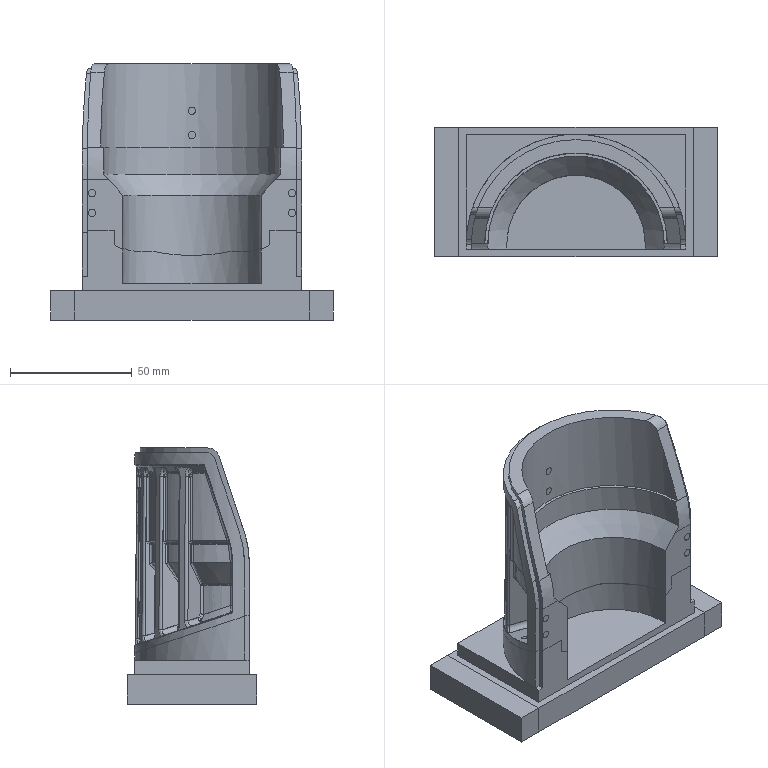NC program | NX | posted by the shop | part box 116 x 53 x 105 mm
Lines 66720 to 68720 of 572762:
T16 M6
;(T16:J-D16  D=16. R=0.)
;(XY=0.2mm Z=0.2mm)
G54 G90 D1
G0 A0.0 C=DC(0.0)
CYCLE832(0.32,_ROUGH,1.)
G0 X-53.306 Y-11.726 S4000 M3 M8
Z3.4
Z.476
G1 Z0.0 F500.
X-50.36 Y-12.824
X-47.214 Y-13.0429
X-44.118 Y-12.441
X-41.284 Y-11.058
X-38.905 Y-8.988
X-37.214 Y-6.338
X-35.878 Y-3.513
X-34.337 Y-.794
X-32.599 Y1.802
X-29.645 Y5.522
X-26.241 Y8.84
X-22.469 Y11.732
X-18.382 Y14.157
X-14.036 Y16.0824
X-9.493 Y17.48
X-4.817 Y18.331
X-.073 Y18.622
X4.672 Y18.351
X9.352 Y17.52
X13.9 Y16.141
X18.254 Y14.235
X22.352 Y11.826
X26.136 Y8.95
X29.553 Y5.647
X32.556 Y1.963
X35.067 Y-2.07
X37.226 Y-6.338
X38.933 Y-8.978
X41.325 Y-11.033
X44.167 Y-12.399
X47.266 Y-12.9826
X50.411 Y-12.744
X53.35 Y-11.629
Z.468
G0 Z3.4
CYCLE832()
;(T16:J-D16  D=16. R=0.)
;(XY=0.3mm Z=0.mm)
SUPA G0 Z-1. D0
SUPA G0 X-1.0 Y-1.0
G54 G90 D1
CYCLE832(0.04,_TOP_SURFACE_SMOOTH_ON+_ORI_SEMIFIN,1.)
TRAFOOF
CYCLE800(0,"AFMING",100000,57,0.,0.,0.,90.,-0.,-180.,0.,0.,0.,-1,100.,1)
G0 X-62.6 Y84.699 S4000 M3
Z102.5121
X-62.6 Y84.699 Z102.5121
Z23.5
G1 X-53. F500.
X53.
Y79.
X50.753 Y76.997
X-50.753
Y69.295
X50.753
Y61.593
X-50.753
Y53.891
X50.753
X60.353
G0 Z102.5121
CYCLE800()
CYCLE832()
;(T16:J-D16  D=16. R=0.)
;(XY=0.3mm Z=0.mm)
SUPA G0 Z-1. D0
SUPA G0 X-1.0 Y-1.0
G54 G90 D1
CYCLE832(0.04,_TOP_SURFACE_SMOOTH_ON+_ORI_SEMIFIN,1.)
TRAFOOF
CYCLE800(0,"AFMING",100000,57,0.,0.,0.,-90.,0.,-0.,0.,0.,0.,-1,100.,1)
G0 X62.6 Y79.001 S4000 M3
Z102.4879
X62.6 Y79.001 Z102.4879
Z23.5
G1 X53. F500.
X-53.
Y84.7
X53.
X62.6
G0 Z102.4879
CYCLE800()
CYCLE832()
;(T16:J-D16  D=16. R=0.)
;(XY=0.3mm Z=0.mm)
SUPA G0 Z-1. D0
SUPA G0 X-1.0 Y-1.0
G54 G90 D1
CYCLE832(0.04,_TOP_SURFACE_SMOOTH_ON+_ORI_SEMIFIN,1.)
TRAFOOF
CYCLE800(0,"AFMING",100000,57,0.,0.,0.,-0.,90.,-90.,0.,0.,0.,-1,100.,1)
G0 X41.1 Y79.001 S4000 M3
Z102.5
X41.1 Y79.001 Z102.5
Z45.
G1 X31.5 F500.
X-31.5
Y84.7
X31.5
X41.1
G0 Z102.5
CYCLE800()
CYCLE832()
;(T16:J-D16  D=16. R=0.)
;(XY=0.3mm Z=0.mm)
SUPA G0 Z-1. D0
SUPA G0 X-1.0 Y-1.0
G54 G90 D1
CYCLE832(0.04,_TOP_SURFACE_SMOOTH_ON+_ORI_SEMIFIN,1.)
TRAFOOF
CYCLE800(0,"AFMING",100000,57,0.,0.,0.,-0.,-90.,90.,0.,0.,0.,-1,100.,1)
G0 X41.1 Y79.001 S4000 M3
Z102.5
X41.1 Y79.001 Z102.5
Z45.
G1 X31.5 F500.
X-31.5
Y84.7
X31.5
X41.1
G0 Z102.5
CYCLE800()
CYCLE832()
;(T16:J-D16  D=16. R=0.)
;(XY=-0.02mm Z=0.mm)
SUPA G0 Z-1. D0
SUPA G0 X-1.0 Y-1.0
G54 G90 D1
G0 A0.0 C=DC(0.0)
CYCLE832(0.002,_TOP_SURFACE_SMOOTH_ON+_ORI_FINISH,1.)
TRAFOOF
G0 X25.429 Y-24.199 S2000 M3
Z35.
Z-33.6151
G1 Z-34.1151 F250.
G41 X26.415 Y-24.368
X26.567 Y-24.364
X26.718 Y-24.352
X26.869 Y-24.332
X27.018 Y-24.304
X27.166 Y-24.269
X27.3122 Y-24.227
X27.4558 Y-24.177
X27.597 Y-24.12
X27.735 Y-24.055
X27.8689 Y-23.984
X28. Y-23.907
X28.126 Y-23.822
X28.248 Y-23.732
X28.365 Y-23.635
X28.478 Y-23.533
X28.585 Y-23.425
X28.686 Y-23.3112
X28.782 Y-23.193
X28.8709 Y-23.07
X28.954 Y-22.943
X29.03 Y-22.811
X29.1001 Y-22.676
X29.163 Y-22.538
X29.219 Y-22.396
X29.267 Y-22.252
X29.308 Y-22.106
X29.342 Y-21.957
X29.3678 Y-21.8077
X29.386 Y-21.6568
X29.397 Y-21.505
X29.4 Y-21.353
X29.394 Y-20.874 F400.
X29.3797 Y-20.394
X29.358 Y-19.915
X29.328 Y-19.437
X29.29 Y-18.959
X29.245 Y-18.481
X29.192 Y-18.005
X29.1311 Y-17.529
X29.062 Y-17.054
X28.986 Y-16.581
X28.902 Y-16.109
X28.81 Y-15.638
X28.7108 Y-15.169
X28.604 Y-14.702
X28.489 Y-14.236
X28.367 Y-13.772
X28.237 Y-13.311
X28.1 Y-12.851
X27.955 Y-12.394
X27.803 Y-11.94
X27.643 Y-11.487
X27.476 Y-11.038
X27.302 Y-10.591
X27.12 Y-10.147
X26.931 Y-9.706
X26.735 Y-9.269
X26.532 Y-8.834
X26.322 Y-8.403
X26.105 Y-7.976
X25.881 Y-7.552
X25.65 Y-7.1315
X25.4125 Y-6.715
X25.168 Y-6.303
X24.917 Y-5.894
X24.659 Y-5.49
X24.395 Y-5.09
X24.124 Y-4.694
X23.846 Y-4.303
X23.563 Y-3.9162
X23.273 Y-3.534
X22.977 Y-3.157
X22.674 Y-2.785
X22.366 Y-2.417
X22.052 Y-2.055
X21.732 Y-1.6981
X21.406 Y-1.3463
X21.074 Y-1.
X20.737 Y-.659
X20.395 Y-.323
X20.047 Y.0064
X19.693 Y.3305
X19.334 Y.649
X18.971 Y.961
X18.602 Y1.268
X18.228 Y1.568
X17.849 Y1.862
X17.466 Y2.15
X17.078 Y2.432
X16.685 Y2.707
X16.288 Y2.976
X15.887 Y3.239
X15.481 Y3.494
X15.072 Y3.744
X14.658 Y3.986
X14.24 Y4.222
X13.819 Y4.451
X13.394 Y4.672
X12.965 Y4.887
X12.533 Y5.095
X12.098 Y5.296
X11.659 Y5.49
X11.217 Y5.677
X10.772 Y5.856
X10.325 Y6.028
X9.874 Y6.193
X9.422 Y6.35
X8.966 Y6.5
X8.508 Y6.6425
X8.048 Y6.778
X7.586 Y6.905
X7.121 Y7.025
X6.6553 Y7.137
X6.187 Y7.242
X5.718 Y7.339
X5.247 Y7.429
X4.774 Y7.51
X4.3 Y7.5843
X3.8254 Y7.651
X3.349 Y7.709
X2.873 Y7.76
X2.395 Y7.803
X1.917 Y7.838
X1.438 Y7.865
X.9589 Y7.885
X.48 Y7.897
X0.0 Y7.9
X-.48 Y7.897
X-.9589 Y7.885
X-1.438 Y7.865
X-1.917 Y7.838
X-2.395 Y7.803
X-2.873 Y7.76
X-3.349 Y7.709
X-3.8254 Y7.651
X-4.3 Y7.5843
X-4.774 Y7.51
X-5.247 Y7.429
X-5.718 Y7.339
X-6.187 Y7.242
X-6.6553 Y7.137
X-7.121 Y7.025
X-7.586 Y6.905
X-8.048 Y6.778
X-8.508 Y6.6425
X-8.966 Y6.5
X-9.422 Y6.35
X-9.874 Y6.193
X-10.325 Y6.028
X-10.772 Y5.856
X-11.217 Y5.677
X-11.659 Y5.49
X-12.098 Y5.296
X-12.533 Y5.095
X-12.965 Y4.887
X-13.394 Y4.672
X-13.819 Y4.451
X-14.24 Y4.222
X-14.658 Y3.986
X-15.072 Y3.744
X-15.481 Y3.494
X-15.887 Y3.239
X-16.288 Y2.976
X-16.685 Y2.707
X-17.078 Y2.432
X-17.466 Y2.15
X-17.849 Y1.862
X-18.228 Y1.568
X-18.602 Y1.268
X-18.971 Y.961
X-19.334 Y.649
X-19.693 Y.3305
X-20.047 Y.0064
X-20.395 Y-.323
X-20.737 Y-.659
X-21.074 Y-1.
X-21.406 Y-1.3463
X-21.732 Y-1.6981
X-22.052 Y-2.055
X-22.366 Y-2.417
X-22.674 Y-2.785
X-22.977 Y-3.157
X-23.273 Y-3.534
X-23.563 Y-3.916
X-23.846 Y-4.303
X-24.124 Y-4.694
X-24.395 Y-5.09
X-24.659 Y-5.49
X-24.917 Y-5.894
X-25.168 Y-6.303
X-25.4125 Y-6.715
X-25.65 Y-7.1315
X-25.881 Y-7.552
X-26.105 Y-7.976
X-26.322 Y-8.403
X-26.532 Y-8.834
X-26.735 Y-9.269
X-26.931 Y-9.706
X-27.12 Y-10.147
X-27.302 Y-10.591
X-27.476 Y-11.038
X-27.643 Y-11.487
X-27.803 Y-11.94
X-27.955 Y-12.394
X-28.1 Y-12.851
X-28.237 Y-13.311
X-28.367 Y-13.772
X-28.489 Y-14.236
X-28.604 Y-14.702
X-28.7108 Y-15.169
X-28.81 Y-15.638
X-28.902 Y-16.109
X-28.986 Y-16.581
X-29.062 Y-17.054
X-29.1311 Y-17.529
X-29.192 Y-18.005
X-29.245 Y-18.481
X-29.29 Y-18.959
X-29.328 Y-19.437
X-29.358 Y-19.915
X-29.3797 Y-20.394
X-29.394 Y-20.874
X-29.4 Y-21.353
X-29.397 Y-21.505
X-29.386 Y-21.6568
X-29.3678 Y-21.8077
X-29.342 Y-21.957
X-29.308 Y-22.106
X-29.267 Y-22.252
X-29.219 Y-22.396
X-29.163 Y-22.538
X-29.1001 Y-22.676
X-29.03 Y-22.811
X-28.954 Y-22.943
X-28.8709 Y-23.07
X-28.782 Y-23.193
X-28.686 Y-23.3112
X-28.585 Y-23.425
X-28.478 Y-23.533
X-28.365 Y-23.635
X-28.248 Y-23.732
X-28.126 Y-23.822
X-28. Y-23.907
X-27.8689 Y-23.984
X-27.735 Y-24.055
X-27.597 Y-24.12
X-27.4558 Y-24.177
X-27.3122 Y-24.227
X-27.166 Y-24.269
X-27.018 Y-24.304
X-26.869 Y-24.332
X-26.718 Y-24.352
X-26.567 Y-24.364
X-26.415 Y-24.368
G40 X-25.429 Y-24.199
Z-33.6151
G0 Z35.
X25.429
Z-33.6151
G1 Z-34.1151 F250.
G41 X26.415 Y-24.368
X26.435 Y-24.368
X26.587 Y-24.364
X26.738 Y-24.352
X26.889 Y-24.332
X27.038 Y-24.304
X27.186 Y-24.269
X27.3322 Y-24.226
X27.4758 Y-24.177
X27.617 Y-24.119
X27.755 Y-24.055
X27.8889 Y-23.984
X28.02 Y-23.906
X28.146 Y-23.822
X28.268 Y-23.732
X28.385 Y-23.635
X28.498 Y-23.532
X28.605 Y-23.424
X28.706 Y-23.3111
X28.802 Y-23.193
X28.8909 Y-23.07
X28.974 Y-22.942
X29.05 Y-22.811
X29.1201 Y-22.676
X29.183 Y-22.538
X29.239 Y-22.396
X29.287 Y-22.252
X29.328 Y-22.106
X29.362 Y-21.957
X29.3878 Y-21.8076
X29.406 Y-21.6567
X29.417 Y-21.505
X29.42 Y-21.353
X29.414 Y-20.873 F400.
X29.4 Y-20.394
X29.378 Y-19.914
X29.348 Y-19.435
X29.31 Y-18.957
X29.265 Y-18.479
X29.212 Y-18.002
X29.151 Y-17.526
X29.082 Y-17.051
X29.006 Y-16.578
X28.922 Y-16.105
X28.83 Y-15.634
X28.73 Y-15.165
X28.623 Y-14.697
X28.508 Y-14.231
X28.386 Y-13.767
X28.256 Y-13.305
X28.119 Y-12.846
X27.974 Y-12.388
X27.822 Y-11.933
X27.662 Y-11.481
X27.495 Y-11.0307
X27.32 Y-10.584
X27.139 Y-10.14
X26.95 Y-9.698
X26.754 Y-9.26
X26.55 Y-8.826
X26.34 Y-8.394
X26.123 Y-7.967
X25.899 Y-7.542
X25.6677 Y-7.122
X25.43 Y-6.705
X25.1851 Y-6.292
X24.934 Y-5.883
X24.6757 Y-5.479
X24.411 Y-5.079
X24.14 Y-4.683
X23.863 Y-4.291
X23.579 Y-3.904
X23.289 Y-3.522
X22.992 Y-3.145
X22.69 Y-2.772
X22.381 Y-2.404
X22.067 Y-2.042
X21.747 Y-1.685
X21.421 Y-1.333
X21.089 Y-.986
X20.751 Y-.645
X20.409 Y-.309
X20.06 Y.021
X19.707 Y.345
X19.3476 Y.664
X18.984 Y.976
X18.614 Y1.283
X18.24 Y1.584
X17.861 Y1.878
X17.478 Y2.166
X17.089 Y2.448
X16.697 Y2.724
X16.299 Y2.993
X15.898 Y3.2554
X15.492 Y3.511
X15.082 Y3.761
X14.668 Y4.003
X14.25 Y4.239
X13.828 Y4.468
X13.403 Y4.69
X12.974 Y4.905
X12.542 Y5.113
X12.106 Y5.314
X11.667 Y5.508
X11.225 Y5.695
X10.78 Y5.874
X10.332 Y6.047
X9.8812 Y6.212
X9.428 Y6.369
X8.972 Y6.519
X8.514 Y6.662
X8.054 Y6.797
X7.591 Y6.924
X7.126 Y7.044
X6.66 Y7.157
X6.192 Y7.262
X5.722 Y7.359
X5.2502 Y7.448
X4.777 Y7.53
X4.303 Y7.604
X3.828 Y7.6704
X3.352 Y7.729
X2.875 Y7.78
X2.397 Y7.823
X1.918 Y7.858
X1.439 Y7.885
X.96 Y7.905
X.48 Y7.917
X0.0 Y7.92
X-.48 Y7.917
X-.96 Y7.905
X-1.439 Y7.885
X-1.918 Y7.858
X-2.397 Y7.823
X-2.875 Y7.78
X-3.352 Y7.729
X-3.828 Y7.6704
X-4.303 Y7.604
X-4.777 Y7.53
X-5.2502 Y7.448
X-5.722 Y7.359
X-6.192 Y7.262
X-6.66 Y7.157
X-7.126 Y7.044
X-7.591 Y6.924
X-8.054 Y6.797
X-8.514 Y6.662
X-8.972 Y6.519
X-9.428 Y6.369
X-9.8812 Y6.212
X-10.332 Y6.047
X-10.78 Y5.874
X-11.225 Y5.695
X-11.667 Y5.508
X-12.106 Y5.314
X-12.542 Y5.113
X-12.974 Y4.905
X-13.403 Y4.69
X-13.828 Y4.468
X-14.25 Y4.239
X-14.668 Y4.003
X-15.082 Y3.761
X-15.4918 Y3.511
X-15.898 Y3.2554
X-16.299 Y2.993
X-16.697 Y2.724
X-17.089 Y2.448
X-17.478 Y2.166
X-17.861 Y1.878
X-18.24 Y1.584
X-18.614 Y1.283
X-18.984 Y.976
X-19.3476 Y.664
X-19.707 Y.345
X-20.06 Y.021
X-20.409 Y-.309
X-20.751 Y-.645
X-21.089 Y-.986
X-21.421 Y-1.333
X-21.747 Y-1.685
X-22.067 Y-2.042
X-22.381 Y-2.404
X-22.69 Y-2.772
X-22.992 Y-3.145
X-23.289 Y-3.522
X-23.579 Y-3.904
X-23.863 Y-4.291
X-24.14 Y-4.683
X-24.411 Y-5.079
X-24.6757 Y-5.479
X-24.934 Y-5.883
X-25.1851 Y-6.292
X-25.43 Y-6.705
X-25.6677 Y-7.122
X-25.899 Y-7.542
X-26.123 Y-7.967
X-26.34 Y-8.394
X-26.55 Y-8.826
X-26.754 Y-9.26
X-26.95 Y-9.698
X-27.139 Y-10.14
X-27.32 Y-10.584
X-27.495 Y-11.0307
X-27.662 Y-11.481
X-27.822 Y-11.933
X-27.974 Y-12.388
X-28.119 Y-12.846
X-28.256 Y-13.305
X-28.386 Y-13.767
X-28.508 Y-14.231
X-28.623 Y-14.697
X-28.73 Y-15.165
X-28.83 Y-15.634
X-28.922 Y-16.105
X-29.006 Y-16.578
X-29.082 Y-17.051
X-29.151 Y-17.526
X-29.212 Y-18.002
X-29.265 Y-18.479
X-29.31 Y-18.957
X-29.348 Y-19.435
X-29.378 Y-19.914
X-29.4 Y-20.394
X-29.414 Y-20.873
X-29.42 Y-21.353
X-29.417 Y-21.505
X-29.406 Y-21.6567
X-29.3878 Y-21.8076
X-29.362 Y-21.957
X-29.328 Y-22.106
X-29.287 Y-22.252
X-29.239 Y-22.396
X-29.183 Y-22.538
X-29.1201 Y-22.676
X-29.05 Y-22.811
X-28.974 Y-22.942
X-28.8909 Y-23.07
X-28.802 Y-23.193
X-28.706 Y-23.3111
X-28.605 Y-23.424
X-28.498 Y-23.532
X-28.385 Y-23.635
X-28.268 Y-23.732
X-28.146 Y-23.822
X-28.02 Y-23.906
X-27.8889 Y-23.984
X-27.755 Y-24.055
X-27.617 Y-24.119
X-27.4758 Y-24.177
X-27.3322 Y-24.226
X-27.186 Y-24.269
X-27.038 Y-24.304
X-26.889 Y-24.332
X-26.738 Y-24.352
X-26.587 Y-24.364
X-26.435 Y-24.368
X-26.415 Y-24.368
G40 X-25.429 Y-24.199
Z-33.6151
G0 Z35.
CYCLE832()
;(T16:J-D16  D=16. R=0.)
;(XY=-0.02mm Z=0.mm)
G54 G90 D1
G0 A0.0 C=DC(0.0)
CYCLE832(0.002,_TOP_SURFACE_SMOOTH_ON+_ORI_FINISH,1.)
TRAFOOF
G0 X24.029 Y-25.618 S2000 M3
Z35.
Z-44.692
G1 Z-45.192 F250.
G41 X25.003 Y-25.844
X25.155 Y-25.849
X25.307 Y-25.845
X25.4589 Y-25.834
X25.61 Y-25.816
X25.759 Y-25.789
X25.908 Y-25.755
X26.054 Y-25.714
X26.198 Y-25.665
X26.339 Y-25.609
X26.478 Y-25.546
X26.613 Y-25.476
X26.744 Y-25.399
X26.871 Y-25.316
X26.994 Y-25.226
X27.112 Y-25.131
X27.225 Y-25.029
X27.333 Y-24.922
X27.435 Y-24.809
X27.531 Y-24.692
X27.622 Y-24.57
X27.7057 Y-24.443
X27.783 Y-24.312
X27.854 Y-24.178
X27.918 Y-24.04
X27.975 Y-23.899
X28.024 Y-23.755
X28.066 Y-23.609
X28.101 Y-23.461
X28.128 Y-23.311
X28.148 Y-23.161
X28.1596 Y-23.009
X28.181 Y-22.537 F400.
X28.195 Y-22.065
X28.2 Y-21.593
X28.198 Y-21.121
X28.188 Y-20.649
X28.169 Y-20.177
X28.143 Y-19.705
X28.109 Y-19.234
X28.067 Y-18.764
X28.0177 Y-18.294
X27.96 Y-17.826
X27.895 Y-17.3579
X27.821 Y-16.891
X27.7403 Y-16.426
X27.651 Y-15.962
X27.555 Y-15.5
X27.451 Y-15.04
X27.338 Y-14.581
X27.2188 Y-14.124
X27.091 Y-13.669
X26.957 Y-13.217
X26.814 Y-12.766
X26.664 Y-12.319
X26.507 Y-11.874
X26.342 Y-11.431
X26.169 Y-10.991
X25.99 Y-10.555
X25.803 Y-10.121
X25.609 Y-9.69
X25.407 Y-9.263
X25.199 Y-8.84
X24.983 Y-8.419
X24.761 Y-8.003
X24.531 Y-7.59
X24.295 Y-7.181
X24.052 Y-6.777
X23.802 Y-6.376
X23.545 Y-5.979
X23.282 Y-5.587
X23.012 Y-5.2
X22.736 Y-4.817
X22.454 Y-4.438
X22.1648 Y-4.0647
X21.87 Y-3.696
X21.569 Y-3.332
X21.261 Y-2.974
X20.948 Y-2.62
X20.629 Y-2.272
X20.304 Y-1.929
X19.974 Y-1.592
X19.637 Y-1.26
X19.2958 Y-.934
X18.949 Y-.614
X18.596 Y-.3
X18.239 Y.009
X17.876 Y.311
X17.508 Y.607
X17.136 Y.897
X16.758 Y1.181
X16.376 Y1.458
X15.989 Y1.729
X15.598 Y1.994
X15.203 Y2.252
X14.803 Y2.5031
X14.399 Y2.748
X13.991 Y2.985
X13.579 Y3.216
X13.163 Y3.44
X12.743 Y3.657
X12.32 Y3.867
X11.8939 Y4.07
X11.464 Y4.265
X11.031 Y4.454
X10.595 Y4.635
X10.156 Y4.808
X9.714 Y4.9747
X9.269 Y5.134
X8.822 Y5.285
X8.372 Y5.429
X7.92 Y5.5655
X7.466 Y5.694
X7.009 Y5.816
X6.551 Y5.929
X6.0907 Y6.035
X5.629 Y6.133
X5.165 Y6.223
X4.7 Y6.306
X4.234 Y6.381
X3.7666 Y6.448
X3.298 Y6.507
X2.829 Y6.558
X2.358 Y6.602
X1.888 Y6.637
X1.416 Y6.665
X.9443 Y6.685
X.472 Y6.697
X0.0 Y6.7
X-.472 Y6.697
X-.9443 Y6.685
X-1.416 Y6.665
X-1.888 Y6.637
X-2.358 Y6.602
X-2.829 Y6.558
X-3.298 Y6.507
X-3.7666 Y6.448
X-4.234 Y6.381
X-4.7 Y6.306
X-5.165 Y6.223
X-5.629 Y6.133
X-6.0907 Y6.035
X-6.551 Y5.929
X-7.009 Y5.816
X-7.4657 Y5.694
X-7.92 Y5.5655
X-8.372 Y5.429
X-8.822 Y5.285
X-9.269 Y5.134
X-9.714 Y4.9747
X-10.156 Y4.808
X-10.595 Y4.635
X-11.031 Y4.454
X-11.464 Y4.265
X-11.894 Y4.07
X-12.32 Y3.867
X-12.743 Y3.657
X-13.163 Y3.44
X-13.579 Y3.216
X-13.991 Y2.985
X-14.399 Y2.748
X-14.803 Y2.503
X-15.203 Y2.252
X-15.598 Y1.994
X-15.989 Y1.729
X-16.376 Y1.4585
X-16.758 Y1.181
X-17.136 Y.897
X-17.508 Y.607
X-17.876 Y.311
X-18.239 Y.009
X-18.596 Y-.3
X-18.949 Y-.614
X-19.296 Y-.934
X-19.637 Y-1.26
X-19.974 Y-1.592
X-20.304 Y-1.929
X-20.629 Y-2.272
X-20.9481 Y-2.62
X-21.2613 Y-2.974
X-21.569 Y-3.332
X-21.87 Y-3.696
X-22.1648 Y-4.065
X-22.454 Y-4.438
X-22.736 Y-4.817
X-23.012 Y-5.2
X-23.282 Y-5.587
X-23.545 Y-5.979
X-23.802 Y-6.376
X-24.052 Y-6.777
X-24.295 Y-7.181
X-24.531 Y-7.59
X-24.761 Y-8.0029
X-24.983 Y-8.419
X-25.199 Y-8.84
X-25.407 Y-9.263
X-25.609 Y-9.69
X-25.803 Y-10.121
X-25.99 Y-10.5546
X-26.169 Y-10.991
X-26.342 Y-11.431
X-26.507 Y-11.874
X-26.664 Y-12.319
X-26.814 Y-12.766
X-26.957 Y-13.217
X-27.091 Y-13.669
X-27.219 Y-14.124
X-27.338 Y-14.5808
X-27.451 Y-15.04
X-27.555 Y-15.5
X-27.651 Y-15.962
X-27.7403 Y-16.426
X-27.821 Y-16.891
X-27.895 Y-17.358
X-27.96 Y-17.826
X-28.0177 Y-18.294
X-28.067 Y-18.764
X-28.109 Y-19.234
X-28.143 Y-19.705
X-28.169 Y-20.177
X-28.188 Y-20.649
X-28.198 Y-21.121
X-28.2 Y-21.593
X-28.195 Y-22.065
X-28.181 Y-22.537
X-28.1596 Y-23.009
X-28.148 Y-23.161
X-28.128 Y-23.311
X-28.101 Y-23.461
X-28.066 Y-23.609
X-28.024 Y-23.755
X-27.975 Y-23.899
X-27.918 Y-24.04
X-27.854 Y-24.178
X-27.7832 Y-24.312
X-27.7057 Y-24.443
X-27.622 Y-24.57
X-27.531 Y-24.692
X-27.435 Y-24.809
X-27.333 Y-24.922
X-27.225 Y-25.029
X-27.112 Y-25.131
X-26.994 Y-25.226
X-26.871 Y-25.316
X-26.744 Y-25.3993
X-26.613 Y-25.476
X-26.478 Y-25.546
X-26.339 Y-25.609
X-26.198 Y-25.665
X-26.054 Y-25.714
X-25.908 Y-25.755
X-25.759 Y-25.789
X-25.61 Y-25.8156
X-25.459 Y-25.834
X-25.307 Y-25.845
X-25.155 Y-25.8489
X-25.003 Y-25.844
G40 X-24.029 Y-25.618
Z-44.692
G0 Z35.
X24.029 Y-25.618
Z-44.692
G1 Z-45.192 F250.
G41 X25.003 Y-25.844
X25.023 Y-25.845
X25.175 Y-25.85
X25.327 Y-25.847
X25.479 Y-25.835
X25.63 Y-25.817
X25.779 Y-25.79
X25.928 Y-25.756
X26.074 Y-25.715
X26.2179 Y-25.666
X26.359 Y-25.6102
X26.498 Y-25.547
X26.6325 Y-25.477
X26.764 Y-25.4
X26.8909 Y-25.317
X27.014 Y-25.227
X27.132 Y-25.132
X27.245 Y-25.03
X27.353 Y-24.923
X27.455 Y-24.81
X27.551 Y-24.6929
X27.642 Y-24.571
X27.726 Y-24.444
X27.803 Y-24.313
X27.874 Y-24.1786
X27.9378 Y-24.041
X27.9946 Y-23.9
X28.044 Y-23.756
X28.086 Y-23.61
X28.121 Y-23.4619
X28.148 Y-23.312
X28.168 Y-23.162
X28.18 Y-23.01
X28.201 Y-22.538 F400.
X28.215 Y-22.066
X28.22 Y-21.593
X28.218 Y-21.12
X28.208 Y-20.648
X28.189 Y-20.176
X28.163 Y-19.704
X28.129 Y-19.233
X28.087 Y-18.762
X28.038 Y-18.292
X27.98 Y-17.823
X27.914 Y-17.355
X27.841 Y-16.888
X27.76 Y-16.423
X27.671 Y-15.958
X27.574 Y-15.496
X27.47 Y-15.035
X27.358 Y-14.576
X27.2381 Y-14.119
X27.111 Y-13.664
X26.976 Y-13.211
X26.833 Y-12.7603
X26.683 Y-12.312
X26.525 Y-11.867
X26.36 Y-11.424
X26.188 Y-10.984
X26.008 Y-10.547
X25.821 Y-10.113
X25.627 Y-9.6821
X25.425 Y-9.255
X25.217 Y-8.831
X25.001 Y-8.41
X24.778 Y-7.993
X24.549 Y-7.58
X24.312 Y-7.1712
X24.069 Y-6.766
X23.819 Y-6.365
X23.562 Y-5.968
X23.2986 Y-5.576
X23.029 Y-5.188
X22.752 Y-4.805
X22.47 Y-4.426
X22.181 Y-4.052
X21.885 Y-3.683
X21.584 Y-3.3194
X21.276 Y-2.961
X20.963 Y-2.607
X20.644 Y-2.258
X20.319 Y-1.916
X19.988 Y-1.578
X19.651 Y-1.246
X19.309 Y-.9199
X18.962 Y-.599
X18.61 Y-.285
X18.252 Y.024
X17.8887 Y.326
X17.521 Y.623
X17.148 Y.913
X16.7701 Y1.197
X16.388 Y1.475
X16.001 Y1.746
X15.609 Y2.011
X15.213 Y2.269
X14.813 Y2.52
X14.409 Y2.7648
X14.001 Y3.003
X13.588 Y3.234
X13.172 Y3.458
X12.752 Y3.675
X12.329 Y3.885
X11.902 Y4.088
X11.4722 Y4.283
X11.039 Y4.472
X10.6024 Y4.653
X10.163 Y4.827
X9.721 Y4.993
X9.276 Y5.153
X8.828 Y5.304
X8.378 Y5.448
X7.926 Y5.5847
X7.471 Y5.714
X7.014 Y5.8349
X6.556 Y5.949
X6.095 Y6.054
X5.633 Y6.153
X5.169 Y6.243
X4.704 Y6.326
X4.237 Y6.401
X3.769 Y6.468
X3.3 Y6.527
X2.831 Y6.578
X2.3601 Y6.622
X1.889 Y6.657
X1.417 Y6.6849
X.945 Y6.705
X.473 Y6.717
X0.0 Y6.72
X-.473 Y6.717
X-.945 Y6.705
X-1.417 Y6.6849
X-1.889 Y6.657
X-2.3601 Y6.622
X-2.831 Y6.578
X-3.3 Y6.527
X-3.769 Y6.468
X-4.237 Y6.401
X-4.704 Y6.326
X-5.169 Y6.243
X-5.633 Y6.153
X-6.095 Y6.054
X-6.556 Y5.949
X-7.014 Y5.8349
X-7.471 Y5.714
X-7.926 Y5.5847
X-8.378 Y5.448
X-8.828 Y5.304
X-9.276 Y5.153
X-9.721 Y4.993
X-10.163 Y4.827
X-10.6024 Y4.653
X-11.039 Y4.472
X-11.4722 Y4.283
X-11.902 Y4.088
X-12.329 Y3.885
X-12.752 Y3.675
X-13.172 Y3.458
X-13.588 Y3.234
X-14.001 Y3.003
X-14.409 Y2.7648
X-14.813 Y2.52
X-15.213 Y2.269
X-15.609 Y2.011
X-16.001 Y1.746
X-16.388 Y1.475
X-16.7701 Y1.197
X-17.148 Y.913
X-17.521 Y.623
X-17.8887 Y.326
X-18.252 Y.024
X-18.61 Y-.285
X-18.962 Y-.599
X-19.309 Y-.9199
X-19.651 Y-1.246
X-19.988 Y-1.578
X-20.319 Y-1.916
X-20.644 Y-2.258
X-20.963 Y-2.607
X-21.276 Y-2.961
X-21.584 Y-3.3194
X-21.885 Y-3.683
X-22.181 Y-4.052
X-22.47 Y-4.426
X-22.752 Y-4.805
X-23.029 Y-5.188
X-23.2986 Y-5.576
X-23.562 Y-5.968
X-23.819 Y-6.365
X-24.069 Y-6.766
X-24.312 Y-7.1712
X-24.549 Y-7.58
X-24.778 Y-7.993
X-25.001 Y-8.41
X-25.217 Y-8.831
X-25.425 Y-9.255
X-25.627 Y-9.6821
X-25.821 Y-10.113
X-26.008 Y-10.547
X-26.188 Y-10.984
X-26.36 Y-11.424
X-26.525 Y-11.867
X-26.683 Y-12.312
X-26.833 Y-12.7603
X-26.976 Y-13.211
X-27.111 Y-13.664
X-27.2381 Y-14.119
X-27.358 Y-14.576
X-27.47 Y-15.035
X-27.574 Y-15.496
X-27.671 Y-15.958
X-27.76 Y-16.423
X-27.841 Y-16.888
X-27.914 Y-17.355
X-27.98 Y-17.823
X-28.038 Y-18.292
X-28.087 Y-18.762
X-28.129 Y-19.233
X-28.163 Y-19.704
X-28.189 Y-20.176
X-28.208 Y-20.648
X-28.218 Y-21.12
X-28.22 Y-21.593
X-28.215 Y-22.066
X-28.201 Y-22.538
X-28.18 Y-23.01
X-28.168 Y-23.162
X-28.148 Y-23.312
X-28.121 Y-23.4619
X-28.086 Y-23.61
X-28.044 Y-23.756
X-27.9946 Y-23.9
X-27.9378 Y-24.041
X-27.874 Y-24.1786
X-27.803 Y-24.313
X-27.726 Y-24.444
X-27.642 Y-24.571
X-27.551 Y-24.6929
X-27.455 Y-24.81
X-27.353 Y-24.923
X-27.245 Y-25.03
X-27.132 Y-25.132
X-27.014 Y-25.227
X-26.8909 Y-25.317
X-26.764 Y-25.4
X-26.6325 Y-25.477
X-26.498 Y-25.547
X-26.359 Y-25.6102
X-26.2179 Y-25.666
X-26.074 Y-25.715
X-25.928 Y-25.756
X-25.779 Y-25.79
X-25.63 Y-25.817
X-25.479 Y-25.835
X-25.327 Y-25.847
X-25.175 Y-25.85
X-25.023 Y-25.845
X-25.003 Y-25.844
G40 X-24.029 Y-25.618
Z-44.692
G0 Z35.
CYCLE832()
;(T16:J-D16  D=16. R=0.)
;(XY=-0.02mm Z=0.mm)
G54 G90 D1
G0 A0.0 C=DC(0.0)
CYCLE832(0.002,_TOP_SURFACE_SMOOTH_ON+_ORI_FINISH,1.)
TRAFOOF
G0 X5.63 Y-36.903 S2000 M3
Z35.
Z-78.467
G1 Z-78.967 F250.
G41 X5.972 Y-37.843
X6.102 Y-38.069
X6.181 Y-38.199
X6.2666 Y-38.324
X6.359 Y-38.445
X6.457 Y-38.561
X6.56 Y-38.673
X6.67 Y-38.778
X6.784 Y-38.878
X6.904 Y-38.972
X7.028 Y-39.06
X7.156 Y-39.142
X7.288 Y-39.217
X7.424 Y-39.285
X7.563 Y-39.346
X7.706 Y-39.4
X7.85 Y-39.4465
X7.997 Y-39.486
X8.146 Y-39.5177
X8.2958 Y-39.542
X8.4469 Y-39.559
X8.599 Y-39.568
X8.751 Y-39.569
X8.903 Y-39.5625
X9.054 Y-39.548
X9.204 Y-39.527
X9.354 Y-39.4973
X9.501 Y-39.46
X9.646 Y-39.416
X9.789 Y-39.365
X9.93 Y-39.3058
X10.067 Y-39.24
X10.2 Y-39.167
X10.544 Y-38.964 F400.
X10.884 Y-38.7546
X11.22 Y-38.538
X11.551 Y-38.315
X11.878 Y-38.086
X12.2 Y-37.85
X12.5178 Y-37.609
X12.831 Y-37.36
X13.139 Y-37.106
X13.4416 Y-36.846
X13.739 Y-36.58
X14.032 Y-36.3083
X14.319 Y-36.031
X14.601 Y-35.748
X14.877 Y-35.459
X15.147 Y-35.165
X15.412 Y-34.866
X15.67 Y-34.562
X15.923 Y-34.253
X16.1696 Y-33.939
X16.41 Y-33.62
X16.644 Y-33.296
X16.872 Y-32.968
X17.093 Y-32.636
X17.308 Y-32.299
X17.516 Y-31.9585
X17.717 Y-31.614
X17.912 Y-31.265
X18.0993 Y-30.913
X18.28 Y-30.556
X18.454 Y-30.197
X18.621 Y-29.834
X18.78 Y-29.468
X18.932 Y-29.099
X19.078 Y-28.727
X19.215 Y-28.352
X19.346 Y-27.975
X19.469 Y-27.595
X19.584 Y-27.213
X19.692 Y-26.828
X19.793 Y-26.442
X19.886 Y-26.053
X19.971 Y-25.663
X20.049 Y-25.272
X20.119 Y-24.879
X20.181 Y-24.484
X20.236 Y-24.089
X20.2824 Y-23.692
X20.321 Y-23.295
X20.353 Y-22.897
X20.376 Y-22.498
X20.392 Y-22.099
X20.4 Y-21.7
Y-21.3
X20.392 Y-20.901
X20.376 Y-20.502
X20.353 Y-20.103
X20.321 Y-19.705
X20.2824 Y-19.308
X20.236 Y-18.911
X20.181 Y-18.516
X20.119 Y-18.121
X20.049 Y-17.728
X19.971 Y-17.337
X19.886 Y-16.947
X19.793 Y-16.558
X19.692 Y-16.172
X19.584 Y-15.787
X19.469 Y-15.405
X19.346 Y-15.025
X19.215 Y-14.648
X19.078 Y-14.273
X18.932 Y-13.901
X18.78 Y-13.532
X18.621 Y-13.166
X18.454 Y-12.803
X18.28 Y-12.444
X18.0993 Y-12.087
X17.912 Y-11.735
X17.717 Y-11.386
X17.516 Y-11.0415
X17.308 Y-10.701
X17.093 Y-10.364
X16.872 Y-10.032
X16.644 Y-9.704
X16.41 Y-9.38
X16.1696 Y-9.061
X15.923 Y-8.747
X15.67 Y-8.438
X15.412 Y-8.134
X15.147 Y-7.835
X14.877 Y-7.541
X14.601 Y-7.252
X14.319 Y-6.969
X14.032 Y-6.6917
X13.739 Y-6.42
X13.4416 Y-6.154
X13.139 Y-5.894
X12.831 Y-5.64
X12.5178 Y-5.391
X12.2 Y-5.15
X11.878 Y-4.914
X11.551 Y-4.685
X11.22 Y-4.462
X10.884 Y-4.2454
X10.544 Y-4.036
X10.2 Y-3.833
X9.8525 Y-3.636
X9.501 Y-3.447
X9.146 Y-3.264
X8.787 Y-3.089
X8.425 Y-2.9205
X8.06 Y-2.759
X7.6915 Y-2.605
X7.3202 Y-2.458
X6.9461 Y-2.318
X6.569 Y-2.186
X6.19 Y-2.061
X5.808 Y-1.944
X5.425 Y-1.834
X5.039 Y-1.732
X4.6507 Y-1.637
X4.261 Y-1.549
X3.87 Y-1.47
X3.477 Y-1.398
X3.083 Y-1.334
X2.688 Y-1.2773
X2.291 Y-1.229
X1.894 Y-1.188
X1.496 Y-1.154
X1.098 Y-1.129
X.699 Y-1.111
X.299 Y-1.1017
X-.1 Y-1.1
X-.499 Y-1.106
X-.898 Y-1.119
X-1.2969 Y-1.141
X-1.695 Y-1.17
X-2.093 Y-1.207
X-2.4895 Y-1.252
X-2.885 Y-1.305
X-3.28 Y-1.365
X-3.674 Y-1.433
X-4.066 Y-1.509
X-4.456 Y-1.592
X-4.845 Y-1.683
X-5.232 Y-1.782
X-5.617 Y-1.888
X-6. Y-2.002
X-6.38 Y-2.1228
X-6.758 Y-2.251
X-7.1335 Y-2.387
X-7.506 Y-2.531
X-7.876 Y-2.681
X-8.243 Y-2.839
X-8.607 Y-3.004
X-8.967 Y-3.176
X-9.324 Y-3.355
X-9.6772 Y-3.541
X-10.027 Y-3.734
X-10.373 Y-3.933
X-10.7145 Y-4.14
X-11.052 Y-4.353
X-11.386 Y-4.572
X-11.715 Y-4.798
X-12.04 Y-5.031
X-12.36 Y-5.27
X-12.675 Y-5.515
X-12.9853 Y-5.766
X-13.291 Y-6.023
X-13.591 Y-6.286
X-13.886 Y-6.555
X-14.176 Y-6.83
X-14.461 Y-7.11
X-14.739 Y-7.396
X-15.013 Y-7.687
X-15.28 Y-7.983
X-15.5418 Y-8.285
X-15.797 Y-8.592
X-16.047 Y-8.904
X-16.291 Y-9.22
X-16.528 Y-9.541
X-16.759 Y-9.867
X-16.983 Y-10.197
X-17.201 Y-10.5318
X-17.413 Y-10.871
X-17.617 Y-11.213
X-17.815 Y-11.5602
X-18.006 Y-11.911
X-18.191 Y-12.265
X-18.368 Y-12.623
X-18.538 Y-12.984
X-18.701 Y-13.349
X-18.857 Y-13.716
X-19.006 Y-14.0867
X-19.147 Y-14.46
X-19.281 Y-14.836
X-19.408 Y-15.215
X-19.527 Y-15.596
X-19.6393 Y-15.9793
X-19.7436 Y-16.365
X-19.84 Y-16.752
X-19.929 Y-17.141
X-20.011 Y-17.5323
X-20.085 Y-17.925
X-20.1509 Y-18.319
X-20.2093 Y-18.714
X-20.26 Y-19.11
X-20.303 Y-19.507
X-20.338 Y-19.904
X-20.365 Y-20.303
X-20.385 Y-20.702
X-20.397 Y-21.101
X-20.4 Y-21.5
X-20.397 Y-21.899
X-20.385 Y-22.298
X-20.365 Y-22.697
X-20.338 Y-23.096
X-20.303 Y-23.493
X-20.26 Y-23.89
X-20.2093 Y-24.286
X-20.1509 Y-24.681
X-20.085 Y-25.075
X-20.011 Y-25.4677
X-19.929 Y-25.859
X-19.84 Y-26.248
X-19.7436 Y-26.635
X-19.6393 Y-27.0207
X-19.527 Y-27.404
X-19.408 Y-27.785
X-19.281 Y-28.164
X-19.147 Y-28.54
X-19.006 Y-28.9133
X-18.857 Y-29.284
X-18.701 Y-29.651
X-18.538 Y-30.016
X-18.368 Y-30.377
X-18.191 Y-30.735
X-18.006 Y-31.089
X-17.815 Y-31.4398
X-17.617 Y-31.787
X-17.413 Y-32.129
X-17.201 Y-32.4682
X-16.983 Y-32.803
X-16.759 Y-33.133
X-16.528 Y-33.459
X-16.291 Y-33.78
X-16.047 Y-34.096
X-15.797 Y-34.408
X-15.5418 Y-34.715
X-15.28 Y-35.017
X-15.013 Y-35.313
X-14.739 Y-35.604
X-14.461 Y-35.89
X-14.176 Y-36.17
X-13.886 Y-36.445
X-13.591 Y-36.714
X-13.291 Y-36.977
X-12.9853 Y-37.234
X-12.675 Y-37.485
X-12.36 Y-37.73
X-12.04 Y-37.969
X-11.715 Y-38.202
X-11.386 Y-38.428
X-11.052 Y-38.647
X-10.7145 Y-38.86
X-10.373 Y-39.067
X-10.027 Y-39.266
X-9.6772 Y-39.459
X-9.324 Y-39.645
X-8.967 Y-39.824
X-8.607 Y-39.996
X-8.243 Y-40.161
X-7.876 Y-40.319
X-7.506 Y-40.469
X-7.1335 Y-40.613
X-6.758 Y-40.749
X-6.38 Y-40.8772
X-6. Y-40.998
X-5.617 Y-41.112
X-5.232 Y-41.218
X-4.845 Y-41.317
X-4.456 Y-41.408
X-4.066 Y-41.491
X-3.674 Y-41.567
X-3.28 Y-41.635
X-2.885 Y-41.695
X-2.4895 Y-41.748
X-2.093 Y-41.793
X-1.695 Y-41.83
X-1.2969 Y-41.859
X-.898 Y-41.881
X-.499 Y-41.894
X-.1 Y-41.9
X.299 Y-41.8983
X.699 Y-41.889
X1.098 Y-41.871
X1.496 Y-41.846
X1.894 Y-41.812
X2.291 Y-41.771
X2.688 Y-41.7227
X3.083 Y-41.666
X3.477 Y-41.602
X3.87 Y-41.53
X4.261 Y-41.451
X4.6507 Y-41.363
X5.039 Y-41.268
X5.425 Y-41.166
X5.808 Y-41.056
X6.19 Y-40.939
X6.569 Y-40.814
X6.9461 Y-40.682
X7.3202 Y-40.542
X7.6915 Y-40.395
X8.06 Y-40.241
X8.425 Y-40.0795
X8.787 Y-39.911
X9.146 Y-39.736
X9.501 Y-39.553
X9.8525 Y-39.364
X10.2 Y-39.167
X10.344 Y-39.083
X10.488 Y-38.998
X10.63 Y-38.912
X10.758 Y-38.83
X10.881 Y-38.741
X11. Y-38.646
X11.114 Y-38.545
X11.222 Y-38.438
X11.325 Y-38.327
X11.422 Y-38.21
X11.513 Y-38.088
X11.598 Y-37.9618
X11.677 Y-37.832
X11.748 Y-37.697
X11.813 Y-37.56
X11.871 Y-37.419
X11.921 Y-37.276
X11.9643 Y-37.13
X12. Y-36.982
X12.028 Y-36.833
X12.049 Y-36.682
X12.0618 Y-36.531
X12.067 Y-36.379
X12.065 Y-36.227
X12.054 Y-36.075
X12.037 Y-35.924
X12.011 Y-35.774
X11.978 Y-35.626
X11.938 Y-35.479
X11.89 Y-35.335
X11.835 Y-35.193
X11.773 Y-35.055
X11.704 Y-34.919
X11.627 Y-34.788
G40 X10.966 Y-34.038
X5.7699 Y-37.146
G41 X6.112 Y-38.086 F250.
X6.191 Y-38.2161
X6.2766 Y-38.3416
X6.369 Y-38.4626
X6.467 Y-38.579
X6.57 Y-38.69
X6.68 Y-38.796
X6.794 Y-38.8955
X6.914 Y-38.99
X7.038 Y-39.077
X7.166 Y-39.159
X7.298 Y-39.234
X7.434 Y-39.302
X7.573 Y-39.363
X7.716 Y-39.417
X7.86 Y-39.464
X8.007 Y-39.503
X8.156 Y-39.535
X8.3058 Y-39.559
X8.4569 Y-39.576
X8.609 Y-39.585
X8.761 Y-39.586
X8.913 Y-39.58
X9.064 Y-39.566
X9.214 Y-39.544
X9.364 Y-39.515
X9.511 Y-39.478
X9.656 Y-39.433
X9.799 Y-39.382
X9.94 Y-39.323
X10.077 Y-39.257
X10.21 Y-39.184
X10.554 Y-38.981 F400.
X10.895 Y-38.772
X11.231 Y-38.555
X11.562 Y-38.3319
X11.889 Y-38.102
X12.212 Y-37.866
X12.53 Y-37.624
X12.843 Y-37.376
X13.152 Y-37.122
X13.455 Y-36.861
X13.753 Y-36.595
X14.046 Y-36.323
X14.3331 Y-36.045
X14.615 Y-35.762
X14.891 Y-35.473
X15.162 Y-35.179
X15.427 Y-34.879
X15.686 Y-34.575
X15.939 Y-34.265
X16.185 Y-33.951
X16.426 Y-33.632
X16.66 Y-33.308
X16.888 Y-32.98
X17.11 Y-32.647
X17.325 Y-32.31
X17.533 Y-31.969
X17.734 Y-31.624
X17.929 Y-31.275
X18.117 Y-30.922
X18.298 Y-30.565
X18.472 Y-30.205
X18.639 Y-29.842
X18.798 Y-29.476
X18.951 Y-29.1064
X19.096 Y-28.734
X19.234 Y-28.359
X19.365 Y-27.9811
X19.488 Y-27.601
X19.604 Y-27.218
X19.7117 Y-26.833
X19.812 Y-26.447
X19.905 Y-26.0579
X19.991 Y-25.667
X20.068 Y-25.275
X20.139 Y-24.882
X20.201 Y-24.487
X20.255 Y-24.091
X20.302 Y-23.694
X20.341 Y-23.296
X20.3726 Y-22.898
X20.396 Y-22.499
X20.4117 Y-22.099
X20.42 Y-21.7
Y-21.3
X20.4117 Y-20.901
X20.396 Y-20.501
X20.3726 Y-20.102
X20.341 Y-19.704
X20.302 Y-19.306
X20.255 Y-18.909
X20.201 Y-18.513
X20.139 Y-18.118
X20.068 Y-17.725
X19.991 Y-17.333
X19.905 Y-16.9421
X19.812 Y-16.553
X19.7117 Y-16.167
X19.604 Y-15.782
X19.488 Y-15.399
X19.365 Y-15.0189
X19.234 Y-14.641
X19.096 Y-14.266
X18.951 Y-13.8936
X18.798 Y-13.524
X18.639 Y-13.158
X18.472 Y-12.795
X18.298 Y-12.435
X18.117 Y-12.078
X17.929 Y-11.725
X17.734 Y-11.376
X17.533 Y-11.031
X17.325 Y-10.69
X17.11 Y-10.353
X16.888 Y-10.02
X16.66 Y-9.692
X16.426 Y-9.368
X16.185 Y-9.049
X15.939 Y-8.735
X15.686 Y-8.425
X15.427 Y-8.121
X15.162 Y-7.821
X14.891 Y-7.527
X14.615 Y-7.238
X14.3331 Y-6.955
X14.046 Y-6.677
X13.753 Y-6.405
X13.455 Y-6.139
X13.152 Y-5.878
X12.843 Y-5.624
X12.53 Y-5.376
X12.212 Y-5.134
X11.889 Y-4.898
X11.562 Y-4.6681
X11.231 Y-4.445
X10.895 Y-4.228
X10.554 Y-4.019
X10.21 Y-3.816
X9.862 Y-3.619
X9.51 Y-3.429
X9.155 Y-3.247
X8.796 Y-3.071
X8.433 Y-2.902
X8.068 Y-2.741
X7.699 Y-2.586
X7.327 Y-2.4394
X6.953 Y-2.3
X6.576 Y-2.167
X6.196 Y-2.042
X5.814 Y-1.925
X5.43 Y-1.815
X5.044 Y-1.712
X4.655 Y-1.617
X4.265 Y-1.5299
X3.874 Y-1.45
X3.48 Y-1.378
X3.086 Y-1.314
X2.69 Y-1.257
X2.293 Y-1.2087
X1.896 Y-1.1677
X1.498 Y-1.134
X1.099 Y-1.109
X.699 Y-1.091
X.3 Y-1.0817
X-.1 Y-1.08
X-.5 Y-1.086
X-.899 Y-1.0993
X-1.298 Y-1.121
X-1.697 Y-1.15
X-2.095 Y-1.187
X-2.492 Y-1.232
X-2.888 Y-1.285
X-3.283 Y-1.345
X-3.677 Y-1.4133
X-4.07 Y-1.489
X-4.46 Y-1.5726
X-4.85 Y-1.664
X-5.237 Y-1.762
X-5.622 Y-1.869
X-6.005 Y-1.983
X-6.386 Y-2.1038
X-6.765 Y-2.233
X-7.14 Y-2.369
X-7.514 Y-2.512
X-7.884 Y-2.663
X-8.251 Y-2.821
X-8.615 Y-2.986
X-8.9757 Y-3.158
X-9.333 Y-3.337
X-9.687 Y-3.523
X-10.037 Y-3.716
X-10.383 Y-3.9161
X-10.725 Y-4.123
X-11.063 Y-4.336
X-11.3969 Y-4.556
X-11.726 Y-4.782
X-12.051 Y-5.015
X-12.372 Y-5.254
X-12.687 Y-5.499
X-12.998 Y-5.75
X-13.3038 Y-6.008
X-13.604 Y-6.271
X-13.9 Y-6.54
X-14.19 Y-6.815
X-14.475 Y-7.0959
X-14.754 Y-7.382
X-15.027 Y-7.673
X-15.295 Y-7.97
X-15.557 Y-8.272
X-15.813 Y-8.5792
X-16.063 Y-8.891
X-16.307 Y-9.208
X-16.544 Y-9.529
X-16.775 Y-9.856
X-17. Y-10.186
X-17.218 Y-10.521
X-17.43 Y-10.86
X-17.6345 Y-11.203
X-17.833 Y-11.55
X-18.024 Y-11.901
X-18.208 Y-12.256
X-18.386 Y-12.614
X-18.556 Y-12.976
X-18.72 Y-13.341
X-18.876 Y-13.7085
X-19.025 Y-14.079
X-19.166 Y-14.453
X-19.3 Y-14.83
X-19.427 Y-15.209
X-19.547 Y-15.59
X-19.659 Y-15.974
X-19.763 Y-16.36
X-19.86 Y-16.748
X-19.949 Y-17.137
X-20.031 Y-17.528
X-20.104 Y-17.921
X-20.171 Y-18.3154
X-20.229 Y-18.7108
X-20.28 Y-19.107
X-20.323 Y-19.505
X-20.358 Y-19.903
X-20.3853 Y-20.302
X-20.405 Y-20.701
X-20.417 Y-21.1
X-20.42 Y-21.5
X-20.417 Y-21.9
X-20.405 Y-22.299
X-20.3853 Y-22.698
X-20.358 Y-23.097
X-20.323 Y-23.495
X-20.28 Y-23.893
X-20.229 Y-24.2892
X-20.171 Y-24.6846
X-20.104 Y-25.079
X-20.031 Y-25.472
X-19.949 Y-25.863
X-19.86 Y-26.252
X-19.763 Y-26.64
X-19.659 Y-27.026
X-19.547 Y-27.41
X-19.427 Y-27.791
X-19.3 Y-28.17
X-19.166 Y-28.547
X-19.025 Y-28.921
X-18.876 Y-29.2915
X-18.72 Y-29.659
X-18.556 Y-30.024
X-18.386 Y-30.386
X-18.208 Y-30.744
X-18.024 Y-31.099
X-17.833 Y-31.45
X-17.6345 Y-31.797
X-17.43 Y-32.14
X-17.218 Y-32.479
X-17. Y-32.814
X-16.775 Y-33.144
X-16.544 Y-33.471
X-16.307 Y-33.792
X-16.063 Y-34.109
X-15.813 Y-34.4208
X-15.557 Y-34.728
X-15.295 Y-35.03
X-15.027 Y-35.327
X-14.754 Y-35.618
X-14.475 Y-35.9041
X-14.19 Y-36.185
X-13.9 Y-36.46
X-13.604 Y-36.729
X-13.3038 Y-36.992
X-12.998 Y-37.25
X-12.687 Y-37.501
X-12.372 Y-37.746
X-12.051 Y-37.985
X-11.726 Y-38.218
X-11.3969 Y-38.444
X-11.063 Y-38.664
X-10.725 Y-38.877
X-10.383 Y-39.0839
X-10.037 Y-39.284
X-9.687 Y-39.477
X-9.333 Y-39.663
X-8.9757 Y-39.842
X-8.615 Y-40.014
X-8.251 Y-40.179
X-7.884 Y-40.337
X-7.514 Y-40.488
X-7.14 Y-40.631
X-6.765 Y-40.767
X-6.386 Y-40.8962
X-6.005 Y-41.017
X-5.622 Y-41.131
X-5.237 Y-41.238
X-4.85 Y-41.336
X-4.46 Y-41.4274
X-4.07 Y-41.511
X-3.677 Y-41.5867
X-3.283 Y-41.655
X-2.888 Y-41.715
X-2.492 Y-41.768
X-2.095 Y-41.813
X-1.697 Y-41.85
X-1.298 Y-41.879
X-.899 Y-41.9007
X-.5 Y-41.914
X-.1 Y-41.92
X.3 Y-41.9183
X.699 Y-41.909
X1.099 Y-41.891
X1.498 Y-41.866
X1.896 Y-41.8323
X2.293 Y-41.7913
X2.69 Y-41.743
X3.086 Y-41.686
X3.48 Y-41.622
X3.874 Y-41.55
X4.265 Y-41.4701
X4.655 Y-41.383
X5.044 Y-41.288
X5.43 Y-41.185
X5.814 Y-41.075
X6.196 Y-40.958
X6.576 Y-40.833
X6.953 Y-40.7
X7.327 Y-40.5606
X7.699 Y-40.414
X8.068 Y-40.259
X8.433 Y-40.098
X8.796 Y-39.929
X9.155 Y-39.753
X9.51 Y-39.571
X9.862 Y-39.381
X10.21 Y-39.184
X10.354 Y-39.101
X10.498 Y-39.016
X10.64 Y-38.929
X10.768 Y-38.847
X10.891 Y-38.758
X11.01 Y-38.663
X11.124 Y-38.562
X11.232 Y-38.456
X11.335 Y-38.344
X11.4323 Y-38.227
X11.523 Y-38.1053
X11.608 Y-37.979
X11.687 Y-37.849
X11.758 Y-37.715
X11.823 Y-37.577
X11.881 Y-37.437
X11.931 Y-37.2932
X11.974 Y-37.147
X12.01 Y-37.
X12.0383 Y-36.8503
X12.0589 Y-36.7
X12.072 Y-36.548
X12.077 Y-36.396
X12.075 Y-36.244
X12.065 Y-36.093
X12.047 Y-35.942
X12.021 Y-35.792
X11.988 Y-35.643
X11.948 Y-35.4968
X11.9 Y-35.3525
X11.845 Y-35.211
X11.783 Y-35.072
X11.714 Y-34.937
X11.637 Y-34.805
X11.502 Y-34.583
G40 X10.84 Y-33.833
Z-78.467
G0 Z35.
CYCLE832()
M9
M5
M01
TRAFOOF
SUPA G0 Z-1. D0
SUPA G0 X-1.0 Y-1.0